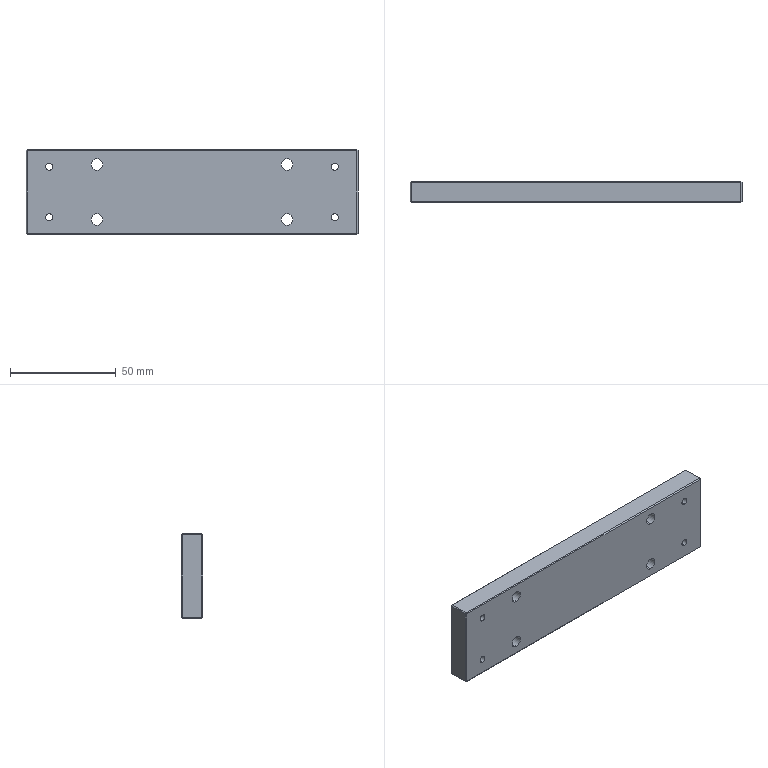Part | STEP file | ND25021-01-JDKM-56-TL | 1 solid | 54 faces | box 157 x 10 x 40 mm | volume 60221 mm3 | plane 30 | cylinder 24 | commonest cylinder face diameters 3.3 x8 5.5 x8 10 x8